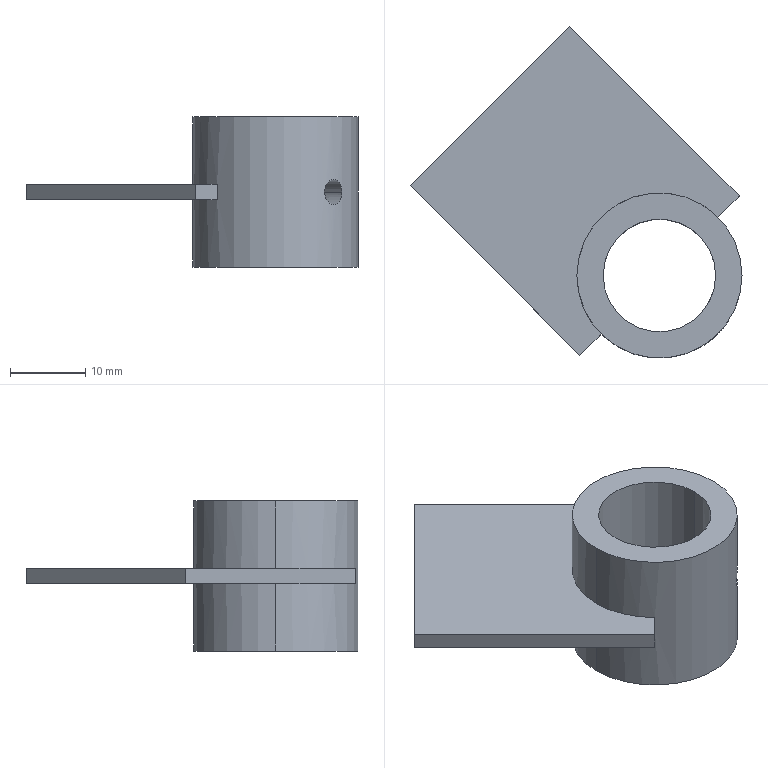Part | SolidWorks | features BaseBody 1 | 1 solid | 15 faces | box 44.234 x 44.234 x 20 mm | volume 5578 mm3 | plane 9 | cylinder 6 | commonest cylinder face diameters 3.3 x2 15 x2 22 x2
STEP:
#1=CARTESIAN_POINT('',(407.047,1579.544,-337.822));
#2=VERTEX_POINT('',#1);
#3=CARTESIAN_POINT('',(429.047,1579.544,-337.822));
#4=VERTEX_POINT('',#3);
#5=CARTESIAN_POINT('',(418.047,1579.544,-337.822));
#6=DIRECTION('',(0.,0.,-1.));
#7=DIRECTION('',(-1.,0.,0.));
#8=AXIS2_PLACEMENT_3D('',#5,#6,#7);
#9=CIRCLE('',#8,11.);
#10=EDGE_CURVE('',#2,#4,#9,.T.);
#11=ORIENTED_EDGE('',*,*,#10,.T.);
#12=CARTESIAN_POINT('',(429.047,1579.544,-357.822));
#13=VERTEX_POINT('',#12);
#14=CARTESIAN_POINT('',(429.047,1579.544,-337.822));
#15=DIRECTION('',(0.,0.,-1.));
#16=VECTOR('',#15,1000.);
#17=LINE('',#14,#16);
#18=EDGE_CURVE('',#4,#13,#17,.T.);
#19=ORIENTED_EDGE('',*,*,#18,.T.);
#20=CARTESIAN_POINT('',(407.047,1579.544,-357.822));
#21=VERTEX_POINT('',#20);
#22=CARTESIAN_POINT('',(418.047,1579.544,-357.822));
#23=DIRECTION('',(0.,0.,1.));
#24=DIRECTION('',(-1.,0.,0.));
#25=AXIS2_PLACEMENT_3D('',#22,#23,#24);
#26=CIRCLE('',#25,11.);
#27=EDGE_CURVE('',#13,#21,#26,.T.);
#28=ORIENTED_EDGE('',*,*,#27,.T.);
#29=CARTESIAN_POINT('',(407.047,1579.544,-348.822));
#30=VERTEX_POINT('',#29);
#31=CARTESIAN_POINT('',(407.047,1579.544,-337.822));
#32=DIRECTION('',(0.,0.,-1.));
#33=VECTOR('',#32,1000.);
#34=LINE('',#31,#33);
#35=EDGE_CURVE('',#30,#21,#34,.T.);
#36=ORIENTED_EDGE('',*,*,#35,.F.);
#37=CARTESIAN_POINT('',(425.825,1587.322,-348.822));
#38=VERTEX_POINT('',#37);
#39=CARTESIAN_POINT('',(418.047,1579.544,-348.822));
#40=DIRECTION('',(0.,0.,-1.));
#41=DIRECTION('',(-1.,0.,0.));
#42=AXIS2_PLACEMENT_3D('',#39,#40,#41);
#43=CIRCLE('',#42,11.);
#44=EDGE_CURVE('',#30,#38,#43,.T.);
#45=ORIENTED_EDGE('',*,*,#44,.T.);
#46=CARTESIAN_POINT('',(425.825,1587.322,-346.822));
#47=VERTEX_POINT('',#46);
#48=CARTESIAN_POINT('',(425.825,1587.322,-348.822));
#49=DIRECTION('',(0.,0.,-1.));
#50=VECTOR('',#49,1000.);
#51=LINE('',#48,#50);
#52=EDGE_CURVE('',#47,#38,#51,.T.);
#53=ORIENTED_EDGE('',*,*,#52,.F.);
#54=CARTESIAN_POINT('',(407.047,1579.544,-346.822));
#55=VERTEX_POINT('',#54);
#56=CARTESIAN_POINT('',(418.047,1579.544,-346.822));
#57=DIRECTION('',(0.,0.,1.));
#58=DIRECTION('',(-1.,0.,0.));
#59=AXIS2_PLACEMENT_3D('',#56,#57,#58);
#60=CIRCLE('',#59,11.);
#61=EDGE_CURVE('',#47,#55,#60,.T.);
#62=ORIENTED_EDGE('',*,*,#61,.T.);
#63=CARTESIAN_POINT('',(407.047,1579.544,-337.822));
#64=DIRECTION('',(0.,0.,-1.));
#65=VECTOR('',#64,1000.);
#66=LINE('',#63,#65);
#67=EDGE_CURVE('',#2,#55,#66,.T.);
#68=ORIENTED_EDGE('',*,*,#67,.F.);
#69=EDGE_LOOP('',(#11,#19,#28,#36,#45,#53,#62,#68));
#70=FACE_OUTER_BOUND('',#69,.T.);
#71=CARTESIAN_POINT('',(418.047,1579.544,-337.822));
#72=DIRECTION('',(0.,0.,-1.));
#73=DIRECTION('',(-1.,0.,0.));
#74=AXIS2_PLACEMENT_3D('',#71,#72,#73);
#75=CYLINDRICAL_SURFACE('',#74,11.);
#76=ADVANCED_FACE('',(#70),#75,.T.);
#77=CARTESIAN_POINT('',(426.903,1573.021,-347.822));
#78=VERTEX_POINT('',#77);
#79=CARTESIAN_POINT('',(424.57,1570.687,-347.822));
#80=VERTEX_POINT('',#79);
#81=CARTESIAN_POINT('',(426.903,1573.021,-347.822));
#82=CARTESIAN_POINT('',(426.903,1573.021,-347.93));
#83=CARTESIAN_POINT('',(426.897,1573.012,-348.04));
#84=CARTESIAN_POINT('',(426.872,1572.977,-348.251));
#85=CARTESIAN_POINT('',(426.853,1572.952,-348.354));
#86=CARTESIAN_POINT('',(426.802,1572.885,-348.554));
#87=CARTESIAN_POINT('',(426.771,1572.844,-348.65));
#88=CARTESIAN_POINT('',(426.697,1572.749,-348.829));
#89=CARTESIAN_POINT('',(426.654,1572.695,-348.912));
#90=CARTESIAN_POINT('',(426.557,1572.574,-349.066));
#91=CARTESIAN_POINT('',(426.504,1572.51,-349.134));
#92=CARTESIAN_POINT('',(426.388,1572.373,-349.254));
#93=CARTESIAN_POINT('',(426.325,1572.3,-349.305));
#94=CARTESIAN_POINT('',(426.125,1572.076,-349.429));
#95=CARTESIAN_POINT('',(425.978,1571.919,-349.473));
#96=CARTESIAN_POINT('',(425.747,1571.688,-349.472));
#97=CARTESIAN_POINT('',(425.67,1571.613,-349.462));
#98=CARTESIAN_POINT('',(425.516,1571.468,-349.419));
#99=CARTESIAN_POINT('',(425.439,1571.397,-349.387));
#100=CARTESIAN_POINT('',(425.289,1571.264,-349.304));
#101=CARTESIAN_POINT('',(425.218,1571.202,-349.254));
#102=CARTESIAN_POINT('',(425.08,1571.086,-349.134));
#103=CARTESIAN_POINT('',(425.015,1571.032,-349.064));
#104=CARTESIAN_POINT('',(424.836,1570.888,-348.836));
#105=CARTESIAN_POINT('',(424.738,1570.813,-348.652));
#106=CARTESIAN_POINT('',(424.605,1570.713,-348.255));
#107=CARTESIAN_POINT('',(424.57,1570.687,-348.038));
#108=CARTESIAN_POINT('',(424.57,1570.687,-347.822));
#109=B_SPLINE_CURVE_WITH_KNOTS('',3,(#81,#82,#83,#84,#85,#86,#87,#88,#89,#90,#91,#92,#93,#94,#95,#96,#97,#98,#99,#100,#101,#102,#103,#104,#105,#106,#107,#108),.UNSPECIFIED.,.F.,.F.,(4,2,2,2,2,2,2,2,2,2,2,2,2,4),(0.002584,0.002906,0.003229,0.003552,0.003875,0.004198,0.00452,0.005166,0.005489,0.005812,0.006134,0.006457,0.007103,0.007748),.UNSPECIFIED.);
#110=EDGE_CURVE('',#78,#80,#109,.T.);
#111=ORIENTED_EDGE('',*,*,#110,.F.);
#112=CARTESIAN_POINT('',(424.387,1575.537,-347.822));
#113=VERTEX_POINT('',#112);
#114=CARTESIAN_POINT('',(419.213,1580.711,-347.822));
#115=DIRECTION('',(-0.7071,0.7071,0.));
#116=VECTOR('',#115,1000.);
#117=LINE('',#114,#116);
#118=EDGE_CURVE('',#78,#113,#117,.T.);
#119=ORIENTED_EDGE('',*,*,#118,.T.);
#120=CARTESIAN_POINT('',(422.053,1573.204,-347.822));
#121=VERTEX_POINT('',#120);
#122=CARTESIAN_POINT('',(422.053,1573.204,-347.822));
#123=CARTESIAN_POINT('',(422.053,1573.204,-347.93));
#124=CARTESIAN_POINT('',(422.063,1573.21,-348.04));
#125=CARTESIAN_POINT('',(422.099,1573.233,-348.252));
#126=CARTESIAN_POINT('',(422.126,1573.25,-348.355));
#127=CARTESIAN_POINT('',(422.233,1573.32,-348.655));
#128=CARTESIAN_POINT('',(422.335,1573.389,-348.836));
#129=CARTESIAN_POINT('',(422.523,1573.526,-349.066));
#130=CARTESIAN_POINT('',(422.59,1573.576,-349.134));
#131=CARTESIAN_POINT('',(422.732,1573.687,-349.253));
#132=CARTESIAN_POINT('',(422.808,1573.748,-349.305));
#133=CARTESIAN_POINT('',(423.037,1573.942,-349.429));
#134=CARTESIAN_POINT('',(423.196,1574.087,-349.473));
#135=CARTESIAN_POINT('',(423.428,1574.319,-349.472));
#136=CARTESIAN_POINT('',(423.502,1574.397,-349.461));
#137=CARTESIAN_POINT('',(423.645,1574.553,-349.419));
#138=CARTESIAN_POINT('',(423.715,1574.632,-349.387));
#139=CARTESIAN_POINT('',(423.844,1574.785,-349.304));
#140=CARTESIAN_POINT('',(423.904,1574.859,-349.253));
#141=CARTESIAN_POINT('',(424.015,1575.001,-349.133));
#142=CARTESIAN_POINT('',(424.066,1575.069,-349.064));
#143=CARTESIAN_POINT('',(424.201,1575.255,-348.836));
#144=CARTESIAN_POINT('',(424.271,1575.359,-348.653));
#145=CARTESIAN_POINT('',(424.363,1575.499,-348.256));
#146=CARTESIAN_POINT('',(424.387,1575.537,-348.038));
#147=CARTESIAN_POINT('',(424.387,1575.537,-347.822));
#148=B_SPLINE_CURVE_WITH_KNOTS('',3,(#122,#123,#124,#125,#126,#127,#128,#129,#130,#131,#132,#133,#134,#135,#136,#137,#138,#139,#140,#141,#142,#143,#144,#145,#146,#147),.UNSPECIFIED.,.F.,.F.,(4,2,2,2,2,2,2,2,2,2,2,2,4),(0.007761,0.008084,0.008408,0.009054,0.009377,0.009701,0.01035,0.01067,0.01099,0.01132,0.01164,0.01229,0.01293),.UNSPECIFIED.);
#149=EDGE_CURVE('',#121,#113,#148,.T.);
#150=ORIENTED_EDGE('',*,*,#149,.F.);
#151=CARTESIAN_POINT('',(416.88,1578.377,-347.822));
#152=DIRECTION('',(-0.7071,0.7071,0.));
#153=VECTOR('',#152,1000.);
#154=LINE('',#151,#153);
#155=EDGE_CURVE('',#80,#121,#154,.T.);
#156=ORIENTED_EDGE('',*,*,#155,.F.);
#157=EDGE_LOOP('',(#111,#119,#150,#156));
#158=FACE_OUTER_BOUND('',#157,.T.);
#159=CARTESIAN_POINT('',(418.047,1579.544,-347.822));
#160=DIRECTION('',(-0.7071,0.7071,0.));
#161=DIRECTION('',(-0.7071,-0.7071,0.));
#162=AXIS2_PLACEMENT_3D('',#159,#160,#161);
#163=CYLINDRICAL_SURFACE('',#162,1.65);
#164=ADVANCED_FACE('',(#158),#163,.F.);
#165=ORIENTED_EDGE('',*,*,#149,.T.);
#166=CARTESIAN_POINT('',(424.387,1575.537,-347.822));
#167=CARTESIAN_POINT('',(424.387,1575.537,-347.714));
#168=CARTESIAN_POINT('',(424.381,1575.528,-347.605));
#169=CARTESIAN_POINT('',(424.357,1575.491,-347.393));
#170=CARTESIAN_POINT('',(424.34,1575.464,-347.29));
#171=CARTESIAN_POINT('',(424.27,1575.358,-346.99));
#172=CARTESIAN_POINT('',(424.201,1575.255,-346.808));
#173=CARTESIAN_POINT('',(424.064,1575.067,-346.579));
#174=CARTESIAN_POINT('',(424.014,1575.,-346.511));
#175=CARTESIAN_POINT('',(423.904,1574.859,-346.391));
#176=CARTESIAN_POINT('',(423.842,1574.783,-346.34));
#177=CARTESIAN_POINT('',(423.649,1574.554,-346.216));
#178=CARTESIAN_POINT('',(423.503,1574.394,-346.172));
#179=CARTESIAN_POINT('',(423.272,1574.162,-346.172));
#180=CARTESIAN_POINT('',(423.194,1574.088,-346.183));
#181=CARTESIAN_POINT('',(423.038,1573.945,-346.226));
#182=CARTESIAN_POINT('',(422.959,1573.876,-346.258));
#183=CARTESIAN_POINT('',(422.806,1573.747,-346.341));
#184=CARTESIAN_POINT('',(422.732,1573.687,-346.391));
#185=CARTESIAN_POINT('',(422.59,1573.576,-346.511));
#186=CARTESIAN_POINT('',(422.521,1573.525,-346.581));
#187=CARTESIAN_POINT('',(422.335,1573.389,-346.808));
#188=CARTESIAN_POINT('',(422.232,1573.32,-346.992));
#189=CARTESIAN_POINT('',(422.091,1573.228,-347.389));
#190=CARTESIAN_POINT('',(422.053,1573.204,-347.606));
#191=CARTESIAN_POINT('',(422.053,1573.204,-347.822));
#192=B_SPLINE_CURVE_WITH_KNOTS('',3,(#166,#167,#168,#169,#170,#171,#172,#173,#174,#175,#176,#177,#178,#179,#180,#181,#182,#183,#184,#185,#186,#187,#188,#189,#190,#191),.UNSPECIFIED.,.F.,.F.,(4,2,2,2,2,2,2,2,2,2,2,2,4),(0.002588,0.002911,0.003235,0.003881,0.004204,0.004528,0.005174,0.005498,0.005821,0.006144,0.006468,0.007114,0.007761),.UNSPECIFIED.);
#193=EDGE_CURVE('',#113,#121,#192,.T.);
#194=ORIENTED_EDGE('',*,*,#193,.T.);
#195=EDGE_LOOP('',(#165,#194));
#196=FACE_BOUND('',#195,.T.);
#197=CARTESIAN_POINT('',(425.547,1579.544,-337.822));
#198=VERTEX_POINT('',#197);
#199=CARTESIAN_POINT('',(410.547,1579.544,-337.822));
#200=VERTEX_POINT('',#199);
#201=CARTESIAN_POINT('',(418.047,1579.544,-337.822));
#202=DIRECTION('',(0.,0.,-1.));
#203=DIRECTION('',(-1.,0.,0.));
#204=AXIS2_PLACEMENT_3D('',#201,#202,#203);
#205=CIRCLE('',#204,7.5);
#206=EDGE_CURVE('',#198,#200,#205,.T.);
#207=ORIENTED_EDGE('',*,*,#206,.F.);
#208=CARTESIAN_POINT('',(425.547,1579.544,-357.822));
#209=VERTEX_POINT('',#208);
#210=CARTESIAN_POINT('',(425.547,1579.544,-337.822));
#211=DIRECTION('',(0.,0.,-1.));
#212=VECTOR('',#211,1000.);
#213=LINE('',#210,#212);
#214=EDGE_CURVE('',#198,#209,#213,.T.);
#215=ORIENTED_EDGE('',*,*,#214,.T.);
#216=CARTESIAN_POINT('',(410.547,1579.544,-357.822));
#217=VERTEX_POINT('',#216);
#218=CARTESIAN_POINT('',(418.047,1579.544,-357.822));
#219=DIRECTION('',(0.,0.,-1.));
#220=DIRECTION('',(-1.,0.,0.));
#221=AXIS2_PLACEMENT_3D('',#218,#219,#220);
#222=CIRCLE('',#221,7.5);
#223=EDGE_CURVE('',#209,#217,#222,.T.);
#224=ORIENTED_EDGE('',*,*,#223,.T.);
#225=CARTESIAN_POINT('',(410.547,1579.544,-337.822));
#226=DIRECTION('',(0.,0.,-1.));
#227=VECTOR('',#226,1000.);
#228=LINE('',#225,#227);
#229=EDGE_CURVE('',#200,#217,#228,.T.);
#230=ORIENTED_EDGE('',*,*,#229,.F.);
#231=EDGE_LOOP('',(#207,#215,#224,#230));
#232=FACE_OUTER_BOUND('',#231,.T.);
#233=CARTESIAN_POINT('',(418.047,1579.544,-337.822));
#234=DIRECTION('',(0.,0.,-1.));
#235=DIRECTION('',(-1.,0.,0.));
#236=AXIS2_PLACEMENT_3D('',#233,#234,#235);
#237=CYLINDRICAL_SURFACE('',#236,7.5);
#238=ADVANCED_FACE('',(#196,#232),#237,.F.);
#239=CARTESIAN_POINT('',(384.813,1591.565,-348.822));
#240=VERTEX_POINT('',#239);
#241=CARTESIAN_POINT('',(407.44,1568.937,-348.822));
#242=VERTEX_POINT('',#241);
#243=CARTESIAN_POINT('',(384.813,1591.565,-348.822));
#244=DIRECTION('',(0.7071,-0.7071,0.));
#245=VECTOR('',#244,1000.);
#246=LINE('',#243,#245);
#247=EDGE_CURVE('',#240,#242,#246,.T.);
#248=ORIENTED_EDGE('',*,*,#247,.F.);
#249=CARTESIAN_POINT('',(406.026,1612.778,-348.822));
#250=VERTEX_POINT('',#249);
#251=CARTESIAN_POINT('',(406.026,1612.778,-348.822));
#252=DIRECTION('',(-0.7071,-0.7071,0.));
#253=VECTOR('',#252,1000.);
#254=LINE('',#251,#253);
#255=EDGE_CURVE('',#250,#240,#254,.T.);
#256=ORIENTED_EDGE('',*,*,#255,.F.);
#257=CARTESIAN_POINT('',(428.653,1590.151,-348.822));
#258=VERTEX_POINT('',#257);
#259=CARTESIAN_POINT('',(428.653,1590.151,-348.822));
#260=DIRECTION('',(-0.7071,0.7071,0.));
#261=VECTOR('',#260,1000.);
#262=LINE('',#259,#261);
#263=EDGE_CURVE('',#258,#250,#262,.T.);
#264=ORIENTED_EDGE('',*,*,#263,.F.);
#265=CARTESIAN_POINT('',(425.825,1587.322,-348.822));
#266=DIRECTION('',(0.7071,0.7071,0.));
#267=VECTOR('',#266,1000.);
#268=LINE('',#265,#267);
#269=EDGE_CURVE('',#38,#258,#268,.T.);
#270=ORIENTED_EDGE('',*,*,#269,.F.);
#271=ORIENTED_EDGE('',*,*,#44,.F.);
#272=CARTESIAN_POINT('',(410.268,1571.766,-348.822));
#273=VERTEX_POINT('',#272);
#274=CARTESIAN_POINT('',(418.047,1579.544,-348.822));
#275=DIRECTION('',(0.,0.,-1.));
#276=DIRECTION('',(-1.,0.,0.));
#277=AXIS2_PLACEMENT_3D('',#274,#275,#276);
#278=CIRCLE('',#277,11.);
#279=EDGE_CURVE('',#273,#30,#278,.T.);
#280=ORIENTED_EDGE('',*,*,#279,.F.);
#281=CARTESIAN_POINT('',(407.44,1568.937,-348.822));
#282=DIRECTION('',(0.7071,0.7071,0.));
#283=VECTOR('',#282,1000.);
#284=LINE('',#281,#283);
#285=EDGE_CURVE('',#242,#273,#284,.T.);
#286=ORIENTED_EDGE('',*,*,#285,.F.);
#287=EDGE_LOOP('',(#248,#256,#264,#270,#271,#280,#286));
#288=FACE_OUTER_BOUND('',#287,.T.);
#289=CARTESIAN_POINT('',(418.047,1579.544,-348.822));
#290=DIRECTION('',(0.,0.,1.));
#291=DIRECTION('',(1.,0.,0.));
#292=AXIS2_PLACEMENT_3D('',#289,#290,#291);
#293=PLANE('',#292);
#294=ADVANCED_FACE('',(#288),#293,.F.);
#295=CARTESIAN_POINT('',(410.268,1571.766,-346.822));
#296=VERTEX_POINT('',#295);
#297=CARTESIAN_POINT('',(410.268,1571.766,-348.822));
#298=DIRECTION('',(0.,0.,1.));
#299=VECTOR('',#298,1000.);
#300=LINE('',#297,#299);
#301=EDGE_CURVE('',#273,#296,#300,.T.);
#302=ORIENTED_EDGE('',*,*,#301,.T.);
#303=CARTESIAN_POINT('',(407.44,1568.937,-346.822));
#304=VERTEX_POINT('',#303);
#305=CARTESIAN_POINT('',(407.44,1568.937,-346.822));
#306=DIRECTION('',(-0.7071,-0.7071,0.));
#307=VECTOR('',#306,1000.);
#308=LINE('',#305,#307);
#309=EDGE_CURVE('',#296,#304,#308,.T.);
#310=ORIENTED_EDGE('',*,*,#309,.T.);
#311=CARTESIAN_POINT('',(407.44,1568.937,-348.822));
#312=DIRECTION('',(0.,0.,-1.));
#313=VECTOR('',#312,1000.);
#314=LINE('',#311,#313);
#315=EDGE_CURVE('',#304,#242,#314,.T.);
#316=ORIENTED_EDGE('',*,*,#315,.T.);
#317=ORIENTED_EDGE('',*,*,#285,.T.);
#318=EDGE_LOOP('',(#302,#310,#316,#317));
#319=FACE_OUTER_BOUND('',#318,.T.);
#320=CARTESIAN_POINT('',(407.44,1568.937,-348.822));
#321=DIRECTION('',(0.7071,-0.7071,0.));
#322=DIRECTION('',(0.7071,0.7071,0.));
#323=AXIS2_PLACEMENT_3D('',#320,#321,#322);
#324=PLANE('',#323);
#325=ADVANCED_FACE('',(#319),#324,.T.);
#326=ORIENTED_EDGE('',*,*,#315,.F.);
#327=CARTESIAN_POINT('',(384.813,1591.565,-346.822));
#328=VERTEX_POINT('',#327);
#329=CARTESIAN_POINT('',(407.44,1568.937,-346.822));
#330=DIRECTION('',(-0.7071,0.7071,0.));
#331=VECTOR('',#330,1000.);
#332=LINE('',#329,#331);
#333=EDGE_CURVE('',#304,#328,#332,.T.);
#334=ORIENTED_EDGE('',*,*,#333,.T.);
#335=CARTESIAN_POINT('',(384.813,1591.565,-348.822));
#336=DIRECTION('',(0.,0.,-1.));
#337=VECTOR('',#336,1000.);
#338=LINE('',#335,#337);
#339=EDGE_CURVE('',#328,#240,#338,.T.);
#340=ORIENTED_EDGE('',*,*,#339,.T.);
#341=ORIENTED_EDGE('',*,*,#247,.T.);
#342=EDGE_LOOP('',(#326,#334,#340,#341));
#343=FACE_OUTER_BOUND('',#342,.T.);
#344=CARTESIAN_POINT('',(407.44,1568.937,-348.822));
#345=DIRECTION('',(-0.7071,-0.7071,0.));
#346=DIRECTION('',(0.7071,-0.7071,0.));
#347=AXIS2_PLACEMENT_3D('',#344,#345,#346);
#348=PLANE('',#347);
#349=ADVANCED_FACE('',(#343),#348,.T.);
#350=ORIENTED_EDGE('',*,*,#339,.F.);
#351=CARTESIAN_POINT('',(406.026,1612.778,-346.822));
#352=VERTEX_POINT('',#351);
#353=CARTESIAN_POINT('',(384.813,1591.565,-346.822));
#354=DIRECTION('',(0.7071,0.7071,0.));
#355=VECTOR('',#354,1000.);
#356=LINE('',#353,#355);
#357=EDGE_CURVE('',#328,#352,#356,.T.);
#358=ORIENTED_EDGE('',*,*,#357,.T.);
#359=CARTESIAN_POINT('',(406.026,1612.778,-348.822));
#360=DIRECTION('',(0.,0.,-1.));
#361=VECTOR('',#360,1000.);
#362=LINE('',#359,#361);
#363=EDGE_CURVE('',#352,#250,#362,.T.);
#364=ORIENTED_EDGE('',*,*,#363,.T.);
#365=ORIENTED_EDGE('',*,*,#255,.T.);
#366=EDGE_LOOP('',(#350,#358,#364,#365));
#367=FACE_OUTER_BOUND('',#366,.T.);
#368=CARTESIAN_POINT('',(384.813,1591.565,-348.822));
#369=DIRECTION('',(-0.7071,0.7071,0.));
#370=DIRECTION('',(-0.7071,-0.7071,0.));
#371=AXIS2_PLACEMENT_3D('',#368,#369,#370);
#372=PLANE('',#371);
#373=ADVANCED_FACE('',(#367),#372,.T.);
#374=ORIENTED_EDGE('',*,*,#363,.F.);
#375=CARTESIAN_POINT('',(428.653,1590.151,-346.822));
#376=VERTEX_POINT('',#375);
#377=CARTESIAN_POINT('',(428.653,1590.151,-346.822));
#378=DIRECTION('',(0.7071,-0.7071,0.));
#379=VECTOR('',#378,1000.);
#380=LINE('',#377,#379);
#381=EDGE_CURVE('',#352,#376,#380,.T.);
#382=ORIENTED_EDGE('',*,*,#381,.T.);
#383=CARTESIAN_POINT('',(428.653,1590.151,-348.822));
#384=DIRECTION('',(0.,0.,-1.));
#385=VECTOR('',#384,1000.);
#386=LINE('',#383,#385);
#387=EDGE_CURVE('',#376,#258,#386,.T.);
#388=ORIENTED_EDGE('',*,*,#387,.T.);
#389=ORIENTED_EDGE('',*,*,#263,.T.);
#390=EDGE_LOOP('',(#374,#382,#388,#389));
#391=FACE_OUTER_BOUND('',#390,.T.);
#392=CARTESIAN_POINT('',(428.653,1590.151,-348.822));
#393=DIRECTION('',(0.7071,0.7071,0.));
#394=DIRECTION('',(-0.7071,0.7071,0.));
#395=AXIS2_PLACEMENT_3D('',#392,#393,#394);
#396=PLANE('',#395);
#397=ADVANCED_FACE('',(#391),#396,.T.);
#398=ORIENTED_EDGE('',*,*,#387,.F.);
#399=CARTESIAN_POINT('',(425.825,1587.322,-346.822));
#400=DIRECTION('',(-0.7071,-0.7071,0.));
#401=VECTOR('',#400,1000.);
#402=LINE('',#399,#401);
#403=EDGE_CURVE('',#376,#47,#402,.T.);
#404=ORIENTED_EDGE('',*,*,#403,.T.);
#405=ORIENTED_EDGE('',*,*,#52,.T.);
#406=ORIENTED_EDGE('',*,*,#269,.T.);
#407=EDGE_LOOP('',(#398,#404,#405,#406));
#408=FACE_OUTER_BOUND('',#407,.T.);
#409=CARTESIAN_POINT('',(425.825,1587.322,-348.822));
#410=DIRECTION('',(0.7071,-0.7071,0.));
#411=DIRECTION('',(0.7071,0.7071,0.));
#412=AXIS2_PLACEMENT_3D('',#409,#410,#411);
#413=PLANE('',#412);
#414=ADVANCED_FACE('',(#408),#413,.T.);
#415=ORIENTED_EDGE('',*,*,#18,.F.);
#416=CARTESIAN_POINT('',(418.047,1579.544,-337.822));
#417=DIRECTION('',(0.,0.,-1.));
#418=DIRECTION('',(-1.,0.,0.));
#419=AXIS2_PLACEMENT_3D('',#416,#417,#418);
#420=CIRCLE('',#419,11.);
#421=EDGE_CURVE('',#4,#2,#420,.T.);
#422=ORIENTED_EDGE('',*,*,#421,.T.);
#423=ORIENTED_EDGE('',*,*,#67,.T.);
#424=CARTESIAN_POINT('',(418.047,1579.544,-346.822));
#425=DIRECTION('',(0.,0.,1.));
#426=DIRECTION('',(-1.,0.,0.));
#427=AXIS2_PLACEMENT_3D('',#424,#425,#426);
#428=CIRCLE('',#427,11.);
#429=EDGE_CURVE('',#55,#296,#428,.T.);
#430=ORIENTED_EDGE('',*,*,#429,.T.);
#431=ORIENTED_EDGE('',*,*,#301,.F.);
#432=ORIENTED_EDGE('',*,*,#279,.T.);
#433=ORIENTED_EDGE('',*,*,#35,.T.);
#434=CARTESIAN_POINT('',(418.047,1579.544,-357.822));
#435=DIRECTION('',(0.,0.,1.));
#436=DIRECTION('',(-1.,0.,0.));
#437=AXIS2_PLACEMENT_3D('',#434,#435,#436);
#438=CIRCLE('',#437,11.);
#439=EDGE_CURVE('',#21,#13,#438,.T.);
#440=ORIENTED_EDGE('',*,*,#439,.T.);
#441=EDGE_LOOP('',(#415,#422,#423,#430,#431,#432,#433,#440));
#442=FACE_OUTER_BOUND('',#441,.T.);
#443=CARTESIAN_POINT('',(424.57,1570.687,-347.822));
#444=CARTESIAN_POINT('',(424.57,1570.687,-347.715));
#445=CARTESIAN_POINT('',(424.579,1570.694,-347.605));
#446=CARTESIAN_POINT('',(424.613,1570.719,-347.393));
#447=CARTESIAN_POINT('',(424.638,1570.738,-347.291));
#448=CARTESIAN_POINT('',(424.705,1570.788,-347.091));
#449=CARTESIAN_POINT('',(424.747,1570.82,-346.994));
#450=CARTESIAN_POINT('',(424.842,1570.894,-346.816));
#451=CARTESIAN_POINT('',(424.896,1570.936,-346.732));
#452=CARTESIAN_POINT('',(425.016,1571.033,-346.579));
#453=CARTESIAN_POINT('',(425.081,1571.086,-346.511));
#454=CARTESIAN_POINT('',(425.217,1571.202,-346.391));
#455=CARTESIAN_POINT('',(425.291,1571.266,-346.339));
#456=CARTESIAN_POINT('',(425.515,1571.465,-346.215));
#457=CARTESIAN_POINT('',(425.671,1571.612,-346.172));
#458=CARTESIAN_POINT('',(425.903,1571.844,-346.172));
#459=CARTESIAN_POINT('',(425.977,1571.921,-346.183));
#460=CARTESIAN_POINT('',(426.122,1572.075,-346.225));
#461=CARTESIAN_POINT('',(426.193,1572.152,-346.257));
#462=CARTESIAN_POINT('',(426.326,1572.301,-346.34));
#463=CARTESIAN_POINT('',(426.388,1572.373,-346.391));
#464=CARTESIAN_POINT('',(426.504,1572.51,-346.511));
#465=CARTESIAN_POINT('',(426.558,1572.576,-346.581));
#466=CARTESIAN_POINT('',(426.702,1572.754,-346.809));
#467=CARTESIAN_POINT('',(426.778,1572.853,-346.993));
#468=CARTESIAN_POINT('',(426.878,1572.985,-347.39));
#469=CARTESIAN_POINT('',(426.903,1573.021,-347.607));
#470=CARTESIAN_POINT('',(426.903,1573.021,-347.822));
#471=B_SPLINE_CURVE_WITH_KNOTS('',3,(#443,#444,#445,#446,#447,#448,#449,#450,#451,#452,#453,#454,#455,#456,#457,#458,#459,#460,#461,#462,#463,#464,#465,#466,#467,#468,#469,#470),.UNSPECIFIED.,.F.,.F.,(4,2,2,2,2,2,2,2,2,2,2,2,2,4),(0.007748,0.008071,0.008394,0.008717,0.009039,0.009362,0.009685,0.01033,0.01065,0.01098,0.0113,0.01162,0.01227,0.01291),.UNSPECIFIED.);
#472=EDGE_CURVE('',#80,#78,#471,.T.);
#473=ORIENTED_EDGE('',*,*,#472,.T.);
#474=ORIENTED_EDGE('',*,*,#110,.T.);
#475=EDGE_LOOP('',(#473,#474));
#476=FACE_BOUND('',#475,.T.);
#477=CARTESIAN_POINT('',(418.047,1579.544,-337.822));
#478=DIRECTION('',(0.,0.,-1.));
#479=DIRECTION('',(-1.,0.,0.));
#480=AXIS2_PLACEMENT_3D('',#477,#478,#479);
#481=CYLINDRICAL_SURFACE('',#480,11.);
#482=ADVANCED_FACE('',(#442,#476),#481,.T.);
#483=ORIENTED_EDGE('',*,*,#309,.F.);
#484=ORIENTED_EDGE('',*,*,#429,.F.);
#485=ORIENTED_EDGE('',*,*,#61,.F.);
#486=ORIENTED_EDGE('',*,*,#403,.F.);
#487=ORIENTED_EDGE('',*,*,#381,.F.);
#488=ORIENTED_EDGE('',*,*,#357,.F.);
#489=ORIENTED_EDGE('',*,*,#333,.F.);
#490=EDGE_LOOP('',(#483,#484,#485,#486,#487,#488,#489));
#491=FACE_OUTER_BOUND('',#490,.T.);
#492=CARTESIAN_POINT('',(418.047,1579.544,-346.822));
#493=DIRECTION('',(0.,0.,1.));
#494=DIRECTION('',(1.,0.,0.));
#495=AXIS2_PLACEMENT_3D('',#492,#493,#494);
#496=PLANE('',#495);
#497=ADVANCED_FACE('',(#491),#496,.T.);
#498=ORIENTED_EDGE('',*,*,#118,.F.);
#499=ORIENTED_EDGE('',*,*,#472,.F.);
#500=ORIENTED_EDGE('',*,*,#155,.T.);
#501=ORIENTED_EDGE('',*,*,#193,.F.);
#502=EDGE_LOOP('',(#498,#499,#500,#501));
#503=FACE_OUTER_BOUND('',#502,.T.);
#504=CARTESIAN_POINT('',(418.047,1579.544,-347.822));
#505=DIRECTION('',(-0.7071,0.7071,0.));
#506=DIRECTION('',(-0.7071,-0.7071,0.));
#507=AXIS2_PLACEMENT_3D('',#504,#505,#506);
#508=CYLINDRICAL_SURFACE('',#507,1.65);
#509=ADVANCED_FACE('',(#503),#508,.F.);
#510=CARTESIAN_POINT('',(418.047,1579.544,-337.822));
#511=DIRECTION('',(0.,0.,-1.));
#512=DIRECTION('',(-1.,0.,0.));
#513=AXIS2_PLACEMENT_3D('',#510,#511,#512);
#514=CIRCLE('',#513,7.5);
#515=EDGE_CURVE('',#200,#198,#514,.T.);
#516=ORIENTED_EDGE('',*,*,#515,.T.);
#517=ORIENTED_EDGE('',*,*,#206,.T.);
#518=EDGE_LOOP('',(#516,#517));
#519=FACE_BOUND('',#518,.T.);
#520=ORIENTED_EDGE('',*,*,#10,.F.);
#521=ORIENTED_EDGE('',*,*,#421,.F.);
#522=EDGE_LOOP('',(#520,#521));
#523=FACE_OUTER_BOUND('',#522,.T.);
#524=CARTESIAN_POINT('',(418.047,1579.544,-337.822));
#525=DIRECTION('',(0.,0.,1.));
#526=DIRECTION('',(1.,0.,0.));
#527=AXIS2_PLACEMENT_3D('',#524,#525,#526);
#528=PLANE('',#527);
#529=ADVANCED_FACE('',(#519,#523),#528,.T.);
#530=CARTESIAN_POINT('',(418.047,1579.544,-357.822));
#531=DIRECTION('',(0.,0.,-1.));
#532=DIRECTION('',(-1.,0.,0.));
#533=AXIS2_PLACEMENT_3D('',#530,#531,#532);
#534=CIRCLE('',#533,7.5);
#535=EDGE_CURVE('',#217,#209,#534,.T.);
#536=ORIENTED_EDGE('',*,*,#535,.F.);
#537=ORIENTED_EDGE('',*,*,#223,.F.);
#538=EDGE_LOOP('',(#536,#537));
#539=FACE_BOUND('',#538,.T.);
#540=ORIENTED_EDGE('',*,*,#439,.F.);
#541=ORIENTED_EDGE('',*,*,#27,.F.);
#542=EDGE_LOOP('',(#540,#541));
#543=FACE_OUTER_BOUND('',#542,.T.);
#544=CARTESIAN_POINT('',(418.047,1579.544,-357.822));
#545=DIRECTION('',(0.,0.,1.));
#546=DIRECTION('',(1.,0.,0.));
#547=AXIS2_PLACEMENT_3D('',#544,#545,#546);
#548=PLANE('',#547);
#549=ADVANCED_FACE('',(#539,#543),#548,.F.);
#550=ORIENTED_EDGE('',*,*,#214,.F.);
#551=ORIENTED_EDGE('',*,*,#515,.F.);
#552=ORIENTED_EDGE('',*,*,#229,.T.);
#553=ORIENTED_EDGE('',*,*,#535,.T.);
#554=EDGE_LOOP('',(#550,#551,#552,#553));
#555=FACE_OUTER_BOUND('',#554,.T.);
#556=CARTESIAN_POINT('',(418.047,1579.544,-337.822));
#557=DIRECTION('',(0.,0.,-1.));
#558=DIRECTION('',(-1.,0.,0.));
#559=AXIS2_PLACEMENT_3D('',#556,#557,#558);
#560=CYLINDRICAL_SURFACE('',#559,7.5);
#561=ADVANCED_FACE('',(#555),#560,.F.);
#562=CLOSED_SHELL('',(#76,#164,#238,#294,#325,#349,#373,#397,#414,#482,#497,#509,#529,#549,#561));
#563=MANIFOLD_SOLID_BREP('',#562);
#564=CARTESIAN_POINT('',(0.,0.,0.));
#565=DIRECTION('',(0.,0.,1.));
#566=DIRECTION('',(1.,0.,0.));
#567=AXIS2_PLACEMENT_3D('',#564,#565,#566);
#568=(LENGTH_UNIT()NAMED_UNIT(*)SI_UNIT(.MILLI.,.METRE.));
#569=UNCERTAINTY_MEASURE_WITH_UNIT(LENGTH_MEASURE(0.00001),#568,'','');
#570=(NAMED_UNIT(*)PLANE_ANGLE_UNIT()SI_UNIT($,.RADIAN.));
#571=(NAMED_UNIT(*)SI_UNIT($,.STERADIAN.)SOLID_ANGLE_UNIT());
#572=(GEOMETRIC_REPRESENTATION_CONTEXT(3)GLOBAL_UNCERTAINTY_ASSIGNED_CONTEXT((#569))GLOBAL_UNIT_ASSIGNED_CONTEXT((#568,#570,#571))REPRESENTATION_CONTEXT('',''));
#573=ADVANCED_BREP_SHAPE_REPRESENTATION('',(#563,#567),#572);